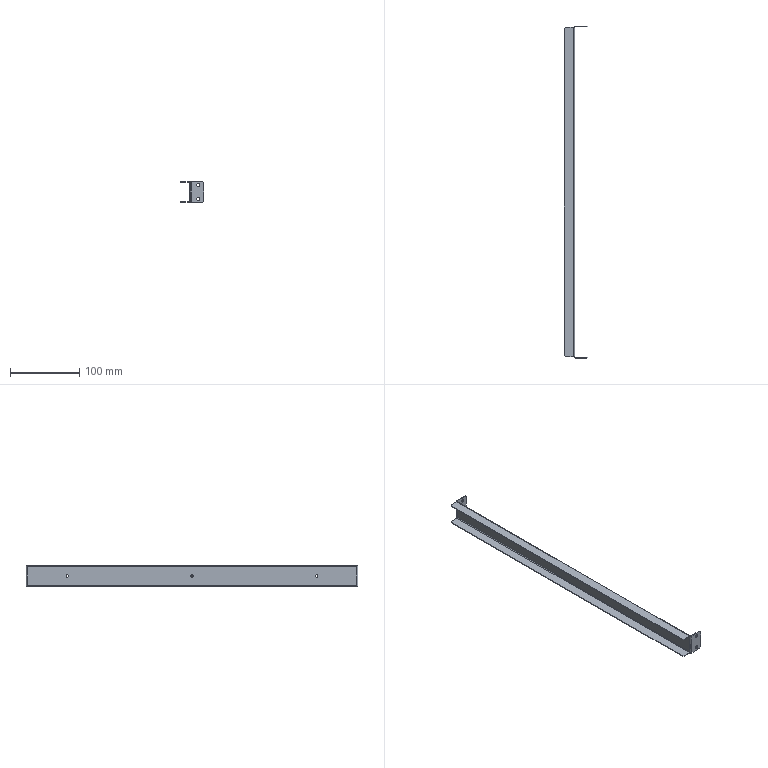Part | SolidWorks | features BaseBody 1 | 1 solid | 56 faces | box 34 x 479 x 30 mm | volume 28054 mm3 | plane 34 | cylinder 22 | commonest cylinder face diameters 4.5 x8 3.3 x6 2 x4 4 x4